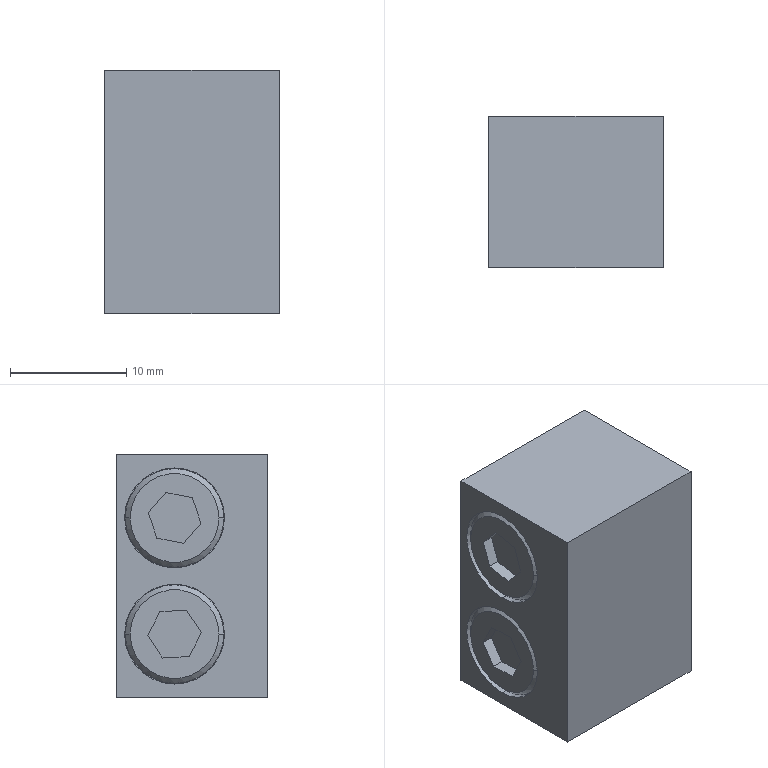Part | NX | 1 solid | 36 faces | box 15 x 13 x 21 mm | volume 4057 mm3 | plane 24 | cylinder 8 | cone 4 | commonest cylinder face diameters 8.5 x4 8.6 x4
STEP:
#1=CARTESIAN_POINT('',(-7.5,-2.325,5.));
#2=VERTEX_POINT('',#1);
#3=CARTESIAN_POINT('',(-7.5,5.325,5.));
#4=VERTEX_POINT('',#3);
#5=CARTESIAN_POINT('',(-7.5,1.5,5.));
#6=DIRECTION('',(-1.,0.,0.));
#7=DIRECTION('',(0.,0.,1.));
#8=AXIS2_PLACEMENT_3D('',#5,#6,#7);
#9=CIRCLE('',#8,3.825);
#10=EDGE_CURVE('',#2,#4,#9,.T.);
#11=ORIENTED_EDGE('',*,*,#10,.F.);
#12=CARTESIAN_POINT('',(-7.075,-2.75,5.));
#13=VERTEX_POINT('',#12);
#14=CARTESIAN_POINT('',(-7.5,-2.325,5.));
#15=DIRECTION('',(0.7071,-0.7071,0.));
#16=VECTOR('',#15,1000.);
#17=LINE('',#14,#16);
#18=EDGE_CURVE('',#13,#2,#17,.F.);
#19=ORIENTED_EDGE('',*,*,#18,.F.);
#20=CARTESIAN_POINT('',(-7.075,1.5,9.25));
#21=VERTEX_POINT('',#20);
#22=CARTESIAN_POINT('',(-7.075,1.5,5.));
#23=DIRECTION('',(1.,0.,0.));
#24=DIRECTION('',(0.,0.,1.));
#25=AXIS2_PLACEMENT_3D('',#22,#23,#24);
#26=CIRCLE('',#25,4.25);
#27=EDGE_CURVE('',#21,#13,#26,.T.);
#28=ORIENTED_EDGE('',*,*,#27,.F.);
#29=CARTESIAN_POINT('',(-7.075,5.75,5.));
#30=VERTEX_POINT('',#29);
#31=CARTESIAN_POINT('',(-7.075,1.5,5.));
#32=DIRECTION('',(1.,0.,0.));
#33=DIRECTION('',(0.,0.,1.));
#34=AXIS2_PLACEMENT_3D('',#31,#32,#33);
#35=CIRCLE('',#34,4.25);
#36=EDGE_CURVE('',#30,#21,#35,.T.);
#37=ORIENTED_EDGE('',*,*,#36,.F.);
#38=CARTESIAN_POINT('',(-7.5,5.325,5.));
#39=DIRECTION('',(0.7071,0.7071,0.));
#40=VECTOR('',#39,1000.);
#41=LINE('',#38,#40);
#42=EDGE_CURVE('',#30,#4,#41,.F.);
#43=ORIENTED_EDGE('',*,*,#42,.T.);
#44=EDGE_LOOP('',(#11,#19,#28,#37,#43));
#45=FACE_BOUND('',#44,.T.);
#46=CARTESIAN_POINT('',(-7.5,1.5,5.));
#47=DIRECTION('',(1.,0.,0.));
#48=DIRECTION('',(0.,-1.,0.));
#49=AXIS2_PLACEMENT_3D('',#46,#47,#48);
#50=CONICAL_SURFACE('',#49,3.825,0.7854);
#51=ADVANCED_FACE('',(#45),#50,.T.);
#52=CARTESIAN_POINT('',(-7.075,1.5,-0.75));
#53=VERTEX_POINT('',#52);
#54=CARTESIAN_POINT('',(-7.075,-2.75,-5.));
#55=VERTEX_POINT('',#54);
#56=CARTESIAN_POINT('',(-7.075,1.5,-5.));
#57=DIRECTION('',(1.,0.,0.));
#58=DIRECTION('',(0.,0.,1.));
#59=AXIS2_PLACEMENT_3D('',#56,#57,#58);
#60=CIRCLE('',#59,4.25);
#61=EDGE_CURVE('',#53,#55,#60,.T.);
#62=ORIENTED_EDGE('',*,*,#61,.F.);
#63=CARTESIAN_POINT('',(-7.075,5.75,-5.));
#64=VERTEX_POINT('',#63);
#65=CARTESIAN_POINT('',(-7.075,1.5,-5.));
#66=DIRECTION('',(1.,0.,0.));
#67=DIRECTION('',(0.,0.,1.));
#68=AXIS2_PLACEMENT_3D('',#65,#66,#67);
#69=CIRCLE('',#68,4.25);
#70=EDGE_CURVE('',#64,#53,#69,.T.);
#71=ORIENTED_EDGE('',*,*,#70,.F.);
#72=CARTESIAN_POINT('',(-7.5,5.325,-5.));
#73=VERTEX_POINT('',#72);
#74=CARTESIAN_POINT('',(-7.5,5.325,-5.));
#75=DIRECTION('',(0.7071,0.7071,0.));
#76=VECTOR('',#75,1000.);
#77=LINE('',#74,#76);
#78=EDGE_CURVE('',#64,#73,#77,.F.);
#79=ORIENTED_EDGE('',*,*,#78,.T.);
#80=CARTESIAN_POINT('',(-7.5,-2.325,-5.));
#81=VERTEX_POINT('',#80);
#82=CARTESIAN_POINT('',(-7.5,1.5,-5.));
#83=DIRECTION('',(-1.,0.,0.));
#84=DIRECTION('',(0.,0.,1.));
#85=AXIS2_PLACEMENT_3D('',#82,#83,#84);
#86=CIRCLE('',#85,3.825);
#87=EDGE_CURVE('',#81,#73,#86,.T.);
#88=ORIENTED_EDGE('',*,*,#87,.F.);
#89=CARTESIAN_POINT('',(-7.5,-2.325,-5.));
#90=DIRECTION('',(0.7071,-0.7071,0.));
#91=VECTOR('',#90,1000.);
#92=LINE('',#89,#91);
#93=EDGE_CURVE('',#55,#81,#92,.F.);
#94=ORIENTED_EDGE('',*,*,#93,.F.);
#95=EDGE_LOOP('',(#62,#71,#79,#88,#94));
#96=FACE_BOUND('',#95,.T.);
#97=CARTESIAN_POINT('',(-7.5,1.5,-5.));
#98=DIRECTION('',(1.,0.,0.));
#99=DIRECTION('',(0.,-1.,0.));
#100=AXIS2_PLACEMENT_3D('',#97,#98,#99);
#101=CONICAL_SURFACE('',#100,3.825,0.7854);
#102=ADVANCED_FACE('',(#96),#101,.T.);
#103=CARTESIAN_POINT('',(-5.5,1.5,9.25));
#104=VERTEX_POINT('',#103);
#105=CARTESIAN_POINT('',(-5.5,1.5,0.75));
#106=VERTEX_POINT('',#105);
#107=CARTESIAN_POINT('',(-5.5,1.5,5.));
#108=DIRECTION('',(-1.,0.,0.));
#109=DIRECTION('',(0.,0.,1.));
#110=AXIS2_PLACEMENT_3D('',#107,#108,#109);
#111=CIRCLE('',#110,4.25);
#112=EDGE_CURVE('',#104,#106,#111,.T.);
#113=ORIENTED_EDGE('',*,*,#112,.T.);
#114=CARTESIAN_POINT('',(-7.075,1.5,0.75));
#115=VERTEX_POINT('',#114);
#116=CARTESIAN_POINT('',(-7.5,1.5,0.75));
#117=DIRECTION('',(1.,0.,0.));
#118=VECTOR('',#117,1000.);
#119=LINE('',#116,#118);
#120=EDGE_CURVE('',#106,#115,#119,.F.);
#121=ORIENTED_EDGE('',*,*,#120,.T.);
#122=CARTESIAN_POINT('',(-7.075,1.5,5.));
#123=DIRECTION('',(1.,0.,0.));
#124=DIRECTION('',(0.,0.,1.));
#125=AXIS2_PLACEMENT_3D('',#122,#123,#124);
#126=CIRCLE('',#125,4.25);
#127=EDGE_CURVE('',#115,#30,#126,.T.);
#128=ORIENTED_EDGE('',*,*,#127,.T.);
#129=ORIENTED_EDGE('',*,*,#36,.T.);
#130=CARTESIAN_POINT('',(-7.5,1.5,9.25));
#131=DIRECTION('',(1.,0.,0.));
#132=VECTOR('',#131,1000.);
#133=LINE('',#130,#132);
#134=EDGE_CURVE('',#104,#21,#133,.F.);
#135=ORIENTED_EDGE('',*,*,#134,.F.);
#136=EDGE_LOOP('',(#113,#121,#128,#129,#135));
#137=FACE_BOUND('',#136,.T.);
#138=CARTESIAN_POINT('',(-7.5,1.5,5.));
#139=DIRECTION('',(1.,0.,0.));
#140=DIRECTION('',(0.,0.,-1.));
#141=AXIS2_PLACEMENT_3D('',#138,#139,#140);
#142=CYLINDRICAL_SURFACE('',#141,4.25);
#143=ADVANCED_FACE('',(#137),#142,.T.);
#144=ORIENTED_EDGE('',*,*,#61,.T.);
#145=CARTESIAN_POINT('',(-7.075,1.5,-9.25));
#146=VERTEX_POINT('',#145);
#147=CARTESIAN_POINT('',(-7.075,1.5,-5.));
#148=DIRECTION('',(1.,0.,0.));
#149=DIRECTION('',(0.,0.,1.));
#150=AXIS2_PLACEMENT_3D('',#147,#148,#149);
#151=CIRCLE('',#150,4.25);
#152=EDGE_CURVE('',#55,#146,#151,.T.);
#153=ORIENTED_EDGE('',*,*,#152,.T.);
#154=CARTESIAN_POINT('',(-5.5,1.5,-9.25));
#155=VERTEX_POINT('',#154);
#156=CARTESIAN_POINT('',(-7.5,1.5,-9.25));
#157=DIRECTION('',(1.,0.,0.));
#158=VECTOR('',#157,1000.);
#159=LINE('',#156,#158);
#160=EDGE_CURVE('',#155,#146,#159,.F.);
#161=ORIENTED_EDGE('',*,*,#160,.F.);
#162=CARTESIAN_POINT('',(-5.5,1.5,-0.75));
#163=VERTEX_POINT('',#162);
#164=CARTESIAN_POINT('',(-5.5,1.5,-5.));
#165=DIRECTION('',(-1.,0.,0.));
#166=DIRECTION('',(0.,0.,-1.));
#167=AXIS2_PLACEMENT_3D('',#164,#165,#166);
#168=CIRCLE('',#167,4.25);
#169=EDGE_CURVE('',#155,#163,#168,.T.);
#170=ORIENTED_EDGE('',*,*,#169,.T.);
#171=CARTESIAN_POINT('',(-7.5,1.5,-0.75));
#172=DIRECTION('',(1.,0.,0.));
#173=VECTOR('',#172,1000.);
#174=LINE('',#171,#173);
#175=EDGE_CURVE('',#163,#53,#174,.F.);
#176=ORIENTED_EDGE('',*,*,#175,.T.);
#177=EDGE_LOOP('',(#144,#153,#161,#170,#176));
#178=FACE_BOUND('',#177,.T.);
#179=CARTESIAN_POINT('',(-7.5,1.5,-5.));
#180=DIRECTION('',(1.,0.,0.));
#181=DIRECTION('',(0.,0.,-1.));
#182=AXIS2_PLACEMENT_3D('',#179,#180,#181);
#183=CYLINDRICAL_SURFACE('',#182,4.25);
#184=ADVANCED_FACE('',(#178),#183,.T.);
#185=CARTESIAN_POINT('',(-7.5,1.5,9.3));
#186=VERTEX_POINT('',#185);
#187=CARTESIAN_POINT('',(-7.5,1.5,0.7));
#188=VERTEX_POINT('',#187);
#189=CARTESIAN_POINT('',(-7.5,1.5,5.));
#190=DIRECTION('',(1.,0.,0.));
#191=DIRECTION('',(0.,0.,1.));
#192=AXIS2_PLACEMENT_3D('',#189,#190,#191);
#193=CIRCLE('',#192,4.3);
#194=EDGE_CURVE('',#186,#188,#193,.T.);
#195=ORIENTED_EDGE('',*,*,#194,.F.);
#196=CARTESIAN_POINT('',(-5.5,1.5,9.3));
#197=VERTEX_POINT('',#196);
#198=CARTESIAN_POINT('',(-5.5,1.5,9.3));
#199=DIRECTION('',(-1.,0.,0.));
#200=VECTOR('',#199,1000.);
#201=LINE('',#198,#200);
#202=EDGE_CURVE('',#197,#186,#201,.T.);
#203=ORIENTED_EDGE('',*,*,#202,.F.);
#204=CARTESIAN_POINT('',(-5.5,1.5,0.7));
#205=VERTEX_POINT('',#204);
#206=CARTESIAN_POINT('',(-5.5,1.5,5.));
#207=DIRECTION('',(1.,0.,0.));
#208=DIRECTION('',(0.,0.,1.));
#209=AXIS2_PLACEMENT_3D('',#206,#207,#208);
#210=CIRCLE('',#209,4.3);
#211=EDGE_CURVE('',#197,#205,#210,.T.);
#212=ORIENTED_EDGE('',*,*,#211,.T.);
#213=CARTESIAN_POINT('',(-5.5,1.5,0.7));
#214=DIRECTION('',(-1.,0.,0.));
#215=VECTOR('',#214,1000.);
#216=LINE('',#213,#215);
#217=EDGE_CURVE('',#205,#188,#216,.T.);
#218=ORIENTED_EDGE('',*,*,#217,.T.);
#219=EDGE_LOOP('',(#195,#203,#212,#218));
#220=FACE_BOUND('',#219,.T.);
#221=CARTESIAN_POINT('',(-5.5,1.5,5.));
#222=DIRECTION('',(-1.,0.,0.));
#223=DIRECTION('',(0.,0.,1.));
#224=AXIS2_PLACEMENT_3D('',#221,#222,#223);
#225=CYLINDRICAL_SURFACE('',#224,4.3);
#226=ADVANCED_FACE('',(#220),#225,.F.);
#227=CARTESIAN_POINT('',(-5.5,1.5,-0.7));
#228=VERTEX_POINT('',#227);
#229=CARTESIAN_POINT('',(-5.5,1.5,-9.3));
#230=VERTEX_POINT('',#229);
#231=CARTESIAN_POINT('',(-5.5,1.5,-5.));
#232=DIRECTION('',(1.,0.,0.));
#233=DIRECTION('',(0.,0.,-1.));
#234=AXIS2_PLACEMENT_3D('',#231,#232,#233);
#235=CIRCLE('',#234,4.3);
#236=EDGE_CURVE('',#228,#230,#235,.T.);
#237=ORIENTED_EDGE('',*,*,#236,.T.);
#238=CARTESIAN_POINT('',(-7.5,1.5,-9.3));
#239=VERTEX_POINT('',#238);
#240=CARTESIAN_POINT('',(-5.5,1.5,-9.3));
#241=DIRECTION('',(-1.,0.,0.));
#242=VECTOR('',#241,1000.);
#243=LINE('',#240,#242);
#244=EDGE_CURVE('',#239,#230,#243,.F.);
#245=ORIENTED_EDGE('',*,*,#244,.F.);
#246=CARTESIAN_POINT('',(-7.5,1.5,-0.7));
#247=VERTEX_POINT('',#246);
#248=CARTESIAN_POINT('',(-7.5,1.5,-5.));
#249=DIRECTION('',(1.,0.,0.));
#250=DIRECTION('',(0.,0.,-1.));
#251=AXIS2_PLACEMENT_3D('',#248,#249,#250);
#252=CIRCLE('',#251,4.3);
#253=EDGE_CURVE('',#247,#239,#252,.T.);
#254=ORIENTED_EDGE('',*,*,#253,.F.);
#255=CARTESIAN_POINT('',(-5.5,1.5,-0.7));
#256=DIRECTION('',(-1.,0.,0.));
#257=VECTOR('',#256,1000.);
#258=LINE('',#255,#257);
#259=EDGE_CURVE('',#247,#228,#258,.F.);
#260=ORIENTED_EDGE('',*,*,#259,.T.);
#261=EDGE_LOOP('',(#237,#245,#254,#260));
#262=FACE_BOUND('',#261,.T.);
#263=CARTESIAN_POINT('',(-5.5,1.5,-5.));
#264=DIRECTION('',(-1.,0.,0.));
#265=DIRECTION('',(0.,0.,1.));
#266=AXIS2_PLACEMENT_3D('',#263,#264,#265);
#267=CYLINDRICAL_SURFACE('',#266,4.3);
#268=ADVANCED_FACE('',(#262),#267,.F.);
#269=CARTESIAN_POINT('',(-5.5,1.5,5.));
#270=DIRECTION('',(1.,0.,0.));
#271=DIRECTION('',(0.,0.,1.));
#272=AXIS2_PLACEMENT_3D('',#269,#270,#271);
#273=CIRCLE('',#272,4.3);
#274=EDGE_CURVE('',#205,#197,#273,.T.);
#275=ORIENTED_EDGE('',*,*,#274,.F.);
#276=ORIENTED_EDGE('',*,*,#211,.F.);
#277=EDGE_LOOP('',(#275,#276));
#278=FACE_BOUND('',#277,.T.);
#279=ORIENTED_EDGE('',*,*,#112,.F.);
#280=CARTESIAN_POINT('',(-5.5,1.5,5.));
#281=DIRECTION('',(-1.,0.,0.));
#282=DIRECTION('',(0.,0.,1.));
#283=AXIS2_PLACEMENT_3D('',#280,#281,#282);
#284=CIRCLE('',#283,4.25);
#285=EDGE_CURVE('',#106,#104,#284,.T.);
#286=ORIENTED_EDGE('',*,*,#285,.F.);
#287=EDGE_LOOP('',(#279,#286));
#288=FACE_BOUND('',#287,.T.);
#289=CARTESIAN_POINT('',(-5.5,1.5,5.));
#290=DIRECTION('',(-1.,0.,0.));
#291=DIRECTION('',(0.,0.,1.));
#292=AXIS2_PLACEMENT_3D('',#289,#290,#291);
#293=PLANE('',#292);
#294=ADVANCED_FACE('',(#278,#288),#293,.T.);
#295=ORIENTED_EDGE('',*,*,#236,.F.);
#296=CARTESIAN_POINT('',(-5.5,1.5,-5.));
#297=DIRECTION('',(1.,0.,0.));
#298=DIRECTION('',(0.,0.,-1.));
#299=AXIS2_PLACEMENT_3D('',#296,#297,#298);
#300=CIRCLE('',#299,4.3);
#301=EDGE_CURVE('',#230,#228,#300,.T.);
#302=ORIENTED_EDGE('',*,*,#301,.F.);
#303=EDGE_LOOP('',(#295,#302));
#304=FACE_BOUND('',#303,.T.);
#305=CARTESIAN_POINT('',(-5.5,1.5,-5.));
#306=DIRECTION('',(-1.,0.,0.));
#307=DIRECTION('',(0.,0.,-1.));
#308=AXIS2_PLACEMENT_3D('',#305,#306,#307);
#309=CIRCLE('',#308,4.25);
#310=EDGE_CURVE('',#163,#155,#309,.T.);
#311=ORIENTED_EDGE('',*,*,#310,.F.);
#312=ORIENTED_EDGE('',*,*,#169,.F.);
#313=EDGE_LOOP('',(#311,#312));
#314=FACE_BOUND('',#313,.T.);
#315=CARTESIAN_POINT('',(-5.5,1.5,-5.));
#316=DIRECTION('',(1.,0.,0.));
#317=DIRECTION('',(0.,1.,0.));
#318=AXIS2_PLACEMENT_3D('',#315,#316,#317);
#319=PLANE('',#318);
#320=ADVANCED_FACE('',(#304,#314),#319,.F.);
#321=CARTESIAN_POINT('',(-7.5,6.5,-10.5));
#322=VERTEX_POINT('',#321);
#323=CARTESIAN_POINT('',(-7.5,-6.5,-10.5));
#324=VERTEX_POINT('',#323);
#325=CARTESIAN_POINT('',(-7.5,6.5,-10.5));
#326=DIRECTION('',(0.,-1.,0.));
#327=VECTOR('',#326,1000.);
#328=LINE('',#325,#327);
#329=EDGE_CURVE('',#322,#324,#328,.T.);
#330=ORIENTED_EDGE('',*,*,#329,.T.);
#331=CARTESIAN_POINT('',(-7.5,-6.5,10.5));
#332=VERTEX_POINT('',#331);
#333=CARTESIAN_POINT('',(-7.5,-6.5,10.5));
#334=DIRECTION('',(0.,0.,-1.));
#335=VECTOR('',#334,1000.);
#336=LINE('',#333,#335);
#337=EDGE_CURVE('',#332,#324,#336,.T.);
#338=ORIENTED_EDGE('',*,*,#337,.F.);
#339=CARTESIAN_POINT('',(-7.5,6.5,10.5));
#340=VERTEX_POINT('',#339);
#341=CARTESIAN_POINT('',(-7.5,6.5,10.5));
#342=DIRECTION('',(0.,-1.,0.));
#343=VECTOR('',#342,1000.);
#344=LINE('',#341,#343);
#345=EDGE_CURVE('',#340,#332,#344,.T.);
#346=ORIENTED_EDGE('',*,*,#345,.F.);
#347=CARTESIAN_POINT('',(-7.5,6.5,10.5));
#348=DIRECTION('',(0.,0.,-1.));
#349=VECTOR('',#348,1000.);
#350=LINE('',#347,#349);
#351=EDGE_CURVE('',#340,#322,#350,.T.);
#352=ORIENTED_EDGE('',*,*,#351,.T.);
#353=EDGE_LOOP('',(#330,#338,#346,#352));
#354=FACE_BOUND('',#353,.T.);
#355=CARTESIAN_POINT('',(-7.5,1.5,-5.));
#356=DIRECTION('',(1.,0.,0.));
#357=DIRECTION('',(0.,0.,-1.));
#358=AXIS2_PLACEMENT_3D('',#355,#356,#357);
#359=CIRCLE('',#358,4.3);
#360=EDGE_CURVE('',#239,#247,#359,.T.);
#361=ORIENTED_EDGE('',*,*,#360,.T.);
#362=ORIENTED_EDGE('',*,*,#253,.T.);
#363=EDGE_LOOP('',(#361,#362));
#364=FACE_BOUND('',#363,.T.);
#365=ORIENTED_EDGE('',*,*,#194,.T.);
#366=CARTESIAN_POINT('',(-7.5,1.5,5.));
#367=DIRECTION('',(1.,0.,0.));
#368=DIRECTION('',(0.,0.,1.));
#369=AXIS2_PLACEMENT_3D('',#366,#367,#368);
#370=CIRCLE('',#369,4.3);
#371=EDGE_CURVE('',#188,#186,#370,.T.);
#372=ORIENTED_EDGE('',*,*,#371,.T.);
#373=EDGE_LOOP('',(#365,#372));
#374=FACE_BOUND('',#373,.T.);
#375=CARTESIAN_POINT('',(-7.5,6.5,10.5));
#376=DIRECTION('',(1.,0.,0.));
#377=DIRECTION('',(0.,1.,0.));
#378=AXIS2_PLACEMENT_3D('',#375,#376,#377);
#379=PLANE('',#378);
#380=ADVANCED_FACE('',(#354,#364,#374),#379,.F.);
#381=CARTESIAN_POINT('',(7.5,-6.5,-10.5));
#382=VERTEX_POINT('',#381);
#383=CARTESIAN_POINT('',(-7.5,-6.5,-10.5));
#384=DIRECTION('',(1.,0.,0.));
#385=VECTOR('',#384,1000.);
#386=LINE('',#383,#385);
#387=EDGE_CURVE('',#324,#382,#386,.T.);
#388=ORIENTED_EDGE('',*,*,#387,.T.);
#389=CARTESIAN_POINT('',(7.5,-6.5,10.5));
#390=VERTEX_POINT('',#389);
#391=CARTESIAN_POINT('',(7.5,-6.5,10.5));
#392=DIRECTION('',(0.,0.,-1.));
#393=VECTOR('',#392,1000.);
#394=LINE('',#391,#393);
#395=EDGE_CURVE('',#390,#382,#394,.T.);
#396=ORIENTED_EDGE('',*,*,#395,.F.);
#397=CARTESIAN_POINT('',(-7.5,-6.5,10.5));
#398=DIRECTION('',(1.,0.,0.));
#399=VECTOR('',#398,1000.);
#400=LINE('',#397,#399);
#401=EDGE_CURVE('',#332,#390,#400,.T.);
#402=ORIENTED_EDGE('',*,*,#401,.F.);
#403=ORIENTED_EDGE('',*,*,#337,.T.);
#404=EDGE_LOOP('',(#388,#396,#402,#403));
#405=FACE_BOUND('',#404,.T.);
#406=CARTESIAN_POINT('',(-7.5,-6.5,10.5));
#407=DIRECTION('',(0.,1.,0.));
#408=DIRECTION('',(1.,0.,0.));
#409=AXIS2_PLACEMENT_3D('',#406,#407,#408);
#410=PLANE('',#409);
#411=ADVANCED_FACE('',(#405),#410,.F.);
#412=CARTESIAN_POINT('',(7.5,6.5,-10.5));
#413=VERTEX_POINT('',#412);
#414=CARTESIAN_POINT('',(7.5,6.5,-10.5));
#415=DIRECTION('',(0.,1.,0.));
#416=VECTOR('',#415,1000.);
#417=LINE('',#414,#416);
#418=EDGE_CURVE('',#382,#413,#417,.T.);
#419=ORIENTED_EDGE('',*,*,#418,.T.);
#420=CARTESIAN_POINT('',(7.5,6.5,10.5));
#421=VERTEX_POINT('',#420);
#422=CARTESIAN_POINT('',(7.5,6.5,10.5));
#423=DIRECTION('',(0.,0.,-1.));
#424=VECTOR('',#423,1000.);
#425=LINE('',#422,#424);
#426=EDGE_CURVE('',#421,#413,#425,.T.);
#427=ORIENTED_EDGE('',*,*,#426,.F.);
#428=CARTESIAN_POINT('',(7.5,6.5,10.5));
#429=DIRECTION('',(0.,1.,0.));
#430=VECTOR('',#429,1000.);
#431=LINE('',#428,#430);
#432=EDGE_CURVE('',#390,#421,#431,.T.);
#433=ORIENTED_EDGE('',*,*,#432,.F.);
#434=ORIENTED_EDGE('',*,*,#395,.T.);
#435=EDGE_LOOP('',(#419,#427,#433,#434));
#436=FACE_BOUND('',#435,.T.);
#437=CARTESIAN_POINT('',(7.5,6.5,10.5));
#438=DIRECTION('',(-1.,0.,0.));
#439=DIRECTION('',(0.,1.,0.));
#440=AXIS2_PLACEMENT_3D('',#437,#438,#439);
#441=PLANE('',#440);
#442=ADVANCED_FACE('',(#436),#441,.F.);
#443=CARTESIAN_POINT('',(-7.5,6.5,-10.5));
#444=DIRECTION('',(-1.,0.,0.));
#445=VECTOR('',#444,1000.);
#446=LINE('',#443,#445);
#447=EDGE_CURVE('',#413,#322,#446,.T.);
#448=ORIENTED_EDGE('',*,*,#447,.T.);
#449=ORIENTED_EDGE('',*,*,#351,.F.);
#450=CARTESIAN_POINT('',(-7.5,6.5,10.5));
#451=DIRECTION('',(-1.,0.,0.));
#452=VECTOR('',#451,1000.);
#453=LINE('',#450,#452);
#454=EDGE_CURVE('',#421,#340,#453,.T.);
#455=ORIENTED_EDGE('',*,*,#454,.F.);
#456=ORIENTED_EDGE('',*,*,#426,.T.);
#457=EDGE_LOOP('',(#448,#449,#455,#456));
#458=FACE_BOUND('',#457,.T.);
#459=CARTESIAN_POINT('',(-7.5,6.5,10.5));
#460=DIRECTION('',(0.,-1.,0.));
#461=DIRECTION('',(0.,0.,-1.));
#462=AXIS2_PLACEMENT_3D('',#459,#460,#461);
#463=PLANE('',#462);
#464=ADVANCED_FACE('',(#458),#463,.F.);
#465=ORIENTED_EDGE('',*,*,#345,.T.);
#466=ORIENTED_EDGE('',*,*,#401,.T.);
#467=ORIENTED_EDGE('',*,*,#432,.T.);
#468=ORIENTED_EDGE('',*,*,#454,.T.);
#469=EDGE_LOOP('',(#465,#466,#467,#468));
#470=FACE_BOUND('',#469,.T.);
#471=CARTESIAN_POINT('',(-7.5,-6.5,10.5));
#472=DIRECTION('',(0.,0.,1.));
#473=DIRECTION('',(1.,0.,0.));
#474=AXIS2_PLACEMENT_3D('',#471,#472,#473);
#475=PLANE('',#474);
#476=ADVANCED_FACE('',(#470),#475,.T.);
#477=ORIENTED_EDGE('',*,*,#329,.F.);
#478=ORIENTED_EDGE('',*,*,#447,.F.);
#479=ORIENTED_EDGE('',*,*,#418,.F.);
#480=ORIENTED_EDGE('',*,*,#387,.F.);
#481=EDGE_LOOP('',(#477,#478,#479,#480));
#482=FACE_BOUND('',#481,.T.);
#483=CARTESIAN_POINT('',(-7.5,-6.5,-10.5));
#484=DIRECTION('',(0.,0.,1.));
#485=DIRECTION('',(1.,0.,0.));
#486=AXIS2_PLACEMENT_3D('',#483,#484,#485);
#487=PLANE('',#486);
#488=ADVANCED_FACE('',(#482),#487,.F.);
#489=CARTESIAN_POINT('',(-7.5,3.766,5.446));
#490=VERTEX_POINT('',#489);
#491=CARTESIAN_POINT('',(-7.5,3.019,3.261));
#492=VERTEX_POINT('',#491);
#493=CARTESIAN_POINT('',(-7.5,3.766,5.446));
#494=DIRECTION('',(0.,-0.3232,-0.9463));
#495=VECTOR('',#494,1000.);
#496=LINE('',#493,#495);
#497=EDGE_CURVE('',#490,#492,#496,.T.);
#498=ORIENTED_EDGE('',*,*,#497,.T.);
#499=CARTESIAN_POINT('',(-6.5,3.019,3.261));
#500=VERTEX_POINT('',#499);
#501=CARTESIAN_POINT('',(-6.5,3.019,3.261));
#502=DIRECTION('',(-1.,0.,0.));
#503=VECTOR('',#502,1000.);
#504=LINE('',#501,#503);
#505=EDGE_CURVE('',#500,#492,#504,.T.);
#506=ORIENTED_EDGE('',*,*,#505,.F.);
#507=CARTESIAN_POINT('',(-6.5,3.766,5.446));
#508=VERTEX_POINT('',#507);
#509=CARTESIAN_POINT('',(-6.5,3.766,5.446));
#510=DIRECTION('',(0.,-0.3232,-0.9463));
#511=VECTOR('',#510,1000.);
#512=LINE('',#509,#511);
#513=EDGE_CURVE('',#508,#500,#512,.T.);
#514=ORIENTED_EDGE('',*,*,#513,.F.);
#515=CARTESIAN_POINT('',(-6.5,3.766,5.446));
#516=DIRECTION('',(-1.,0.,0.));
#517=VECTOR('',#516,1000.);
#518=LINE('',#515,#517);
#519=EDGE_CURVE('',#508,#490,#518,.T.);
#520=ORIENTED_EDGE('',*,*,#519,.T.);
#521=EDGE_LOOP('',(#498,#506,#514,#520));
#522=FACE_BOUND('',#521,.T.);
#523=CARTESIAN_POINT('',(-6.5,3.766,5.446));
#524=DIRECTION('',(0.,0.9463,-0.3232));
#525=DIRECTION('',(-1.,0.,0.));
#526=AXIS2_PLACEMENT_3D('',#523,#524,#525);
#527=PLANE('',#526);
#528=ADVANCED_FACE('',(#522),#527,.F.);
#529=CARTESIAN_POINT('',(-7.5,0.7535,2.815));
#530=VERTEX_POINT('',#529);
#531=CARTESIAN_POINT('',(-7.5,-0.7659,4.554));
#532=VERTEX_POINT('',#531);
#533=CARTESIAN_POINT('',(-7.5,0.7535,2.815));
#534=DIRECTION('',(0.,-0.6579,0.7531));
#535=VECTOR('',#534,1000.);
#536=LINE('',#533,#535);
#537=EDGE_CURVE('',#530,#532,#536,.T.);
#538=ORIENTED_EDGE('',*,*,#537,.T.);
#539=CARTESIAN_POINT('',(-6.5,-0.7659,4.554));
#540=VERTEX_POINT('',#539);
#541=CARTESIAN_POINT('',(-6.5,-0.7659,4.554));
#542=DIRECTION('',(-1.,0.,0.));
#543=VECTOR('',#542,1000.);
#544=LINE('',#541,#543);
#545=EDGE_CURVE('',#540,#532,#544,.T.);
#546=ORIENTED_EDGE('',*,*,#545,.F.);
#547=CARTESIAN_POINT('',(-6.5,0.7535,2.815));
#548=VERTEX_POINT('',#547);
#549=CARTESIAN_POINT('',(-6.5,0.7535,2.815));
#550=DIRECTION('',(0.,-0.6579,0.7531));
#551=VECTOR('',#550,1000.);
#552=LINE('',#549,#551);
#553=EDGE_CURVE('',#548,#540,#552,.T.);
#554=ORIENTED_EDGE('',*,*,#553,.F.);
#555=CARTESIAN_POINT('',(-6.5,0.7535,2.815));
#556=DIRECTION('',(-1.,0.,0.));
#557=VECTOR('',#556,1000.);
#558=LINE('',#555,#557);
#559=EDGE_CURVE('',#548,#530,#558,.T.);
#560=ORIENTED_EDGE('',*,*,#559,.T.);
#561=EDGE_LOOP('',(#538,#546,#554,#560));
#562=FACE_BOUND('',#561,.T.);
#563=CARTESIAN_POINT('',(-6.5,0.7535,2.815));
#564=DIRECTION('',(0.,-0.7531,-0.6579));
#565=DIRECTION('',(0.,0.6579,-0.7531));
#566=AXIS2_PLACEMENT_3D('',#563,#564,#565);
#567=PLANE('',#566);
#568=ADVANCED_FACE('',(#562),#567,.F.);
#569=CARTESIAN_POINT('',(-6.5,-0.01938,6.739));
#570=VERTEX_POINT('',#569);
#571=CARTESIAN_POINT('',(-6.5,-0.7659,4.554));
#572=DIRECTION('',(0.,0.3232,0.9463));
#573=VECTOR('',#572,1000.);
#574=LINE('',#571,#573);
#575=EDGE_CURVE('',#540,#570,#574,.T.);
#576=ORIENTED_EDGE('',*,*,#575,.T.);
#577=CARTESIAN_POINT('',(-6.5,2.246,7.185));
#578=VERTEX_POINT('',#577);
#579=CARTESIAN_POINT('',(-6.5,-0.01938,6.739));
#580=DIRECTION('',(0.,0.9812,0.1932));
#581=VECTOR('',#580,1000.);
#582=LINE('',#579,#581);
#583=EDGE_CURVE('',#570,#578,#582,.T.);
#584=ORIENTED_EDGE('',*,*,#583,.T.);
#585=CARTESIAN_POINT('',(-6.5,2.246,7.185));
#586=DIRECTION('',(0.,0.6579,-0.7531));
#587=VECTOR('',#586,1000.);
#588=LINE('',#585,#587);
#589=EDGE_CURVE('',#578,#508,#588,.T.);
#590=ORIENTED_EDGE('',*,*,#589,.T.);
#591=ORIENTED_EDGE('',*,*,#513,.T.);
#592=CARTESIAN_POINT('',(-6.5,3.019,3.261));
#593=DIRECTION('',(0.,-0.9812,-0.1932));
#594=VECTOR('',#593,1000.);
#595=LINE('',#592,#594);
#596=EDGE_CURVE('',#500,#548,#595,.T.);
#597=ORIENTED_EDGE('',*,*,#596,.T.);
#598=ORIENTED_EDGE('',*,*,#553,.T.);
#599=EDGE_LOOP('',(#576,#584,#590,#591,#597,#598));
#600=FACE_BOUND('',#599,.T.);
#601=CARTESIAN_POINT('',(-6.5,-0.7659,4.554));
#602=DIRECTION('',(1.,0.,0.));
#603=DIRECTION('',(0.,1.,0.));
#604=AXIS2_PLACEMENT_3D('',#601,#602,#603);
#605=PLANE('',#604);
#606=ADVANCED_FACE('',(#600),#605,.F.);
#607=ORIENTED_EDGE('',*,*,#87,.T.);
#608=CARTESIAN_POINT('',(-7.5,1.5,-5.));
#609=DIRECTION('',(-1.,0.,0.));
#610=DIRECTION('',(0.,0.,1.));
#611=AXIS2_PLACEMENT_3D('',#608,#609,#610);
#612=CIRCLE('',#611,3.825);
#613=EDGE_CURVE('',#73,#81,#612,.T.);
#614=ORIENTED_EDGE('',*,*,#613,.T.);
#615=EDGE_LOOP('',(#607,#614));
#616=FACE_BOUND('',#615,.T.);
#617=CARTESIAN_POINT('',(-7.5,0.2336,-6.931));
#618=VERTEX_POINT('',#617);
#619=CARTESIAN_POINT('',(-7.5,-0.8057,-4.869));
#620=VERTEX_POINT('',#619);
#621=CARTESIAN_POINT('',(-7.5,0.2336,-6.931));
#622=DIRECTION('',(0.,-0.45,0.893));
#623=VECTOR('',#622,1000.);
#624=LINE('',#621,#623);
#625=EDGE_CURVE('',#618,#620,#624,.T.);
#626=ORIENTED_EDGE('',*,*,#625,.F.);
#627=CARTESIAN_POINT('',(-7.5,2.539,-7.062));
#628=VERTEX_POINT('',#627);
#629=CARTESIAN_POINT('',(-7.5,2.539,-7.062));
#630=DIRECTION('',(0.,-0.9984,0.05679));
#631=VECTOR('',#630,1000.);
#632=LINE('',#629,#631);
#633=EDGE_CURVE('',#628,#618,#632,.T.);
#634=ORIENTED_EDGE('',*,*,#633,.F.);
#635=CARTESIAN_POINT('',(-7.5,3.806,-5.131));
#636=VERTEX_POINT('',#635);
#637=CARTESIAN_POINT('',(-7.5,3.806,-5.131));
#638=DIRECTION('',(0.,-0.5484,-0.8362));
#639=VECTOR('',#638,1000.);
#640=LINE('',#637,#639);
#641=EDGE_CURVE('',#636,#628,#640,.T.);
#642=ORIENTED_EDGE('',*,*,#641,.F.);
#643=CARTESIAN_POINT('',(-7.5,2.766,-3.069));
#644=VERTEX_POINT('',#643);
#645=CARTESIAN_POINT('',(-7.5,2.766,-3.069));
#646=DIRECTION('',(0.,0.45,-0.893));
#647=VECTOR('',#646,1000.);
#648=LINE('',#645,#647);
#649=EDGE_CURVE('',#644,#636,#648,.T.);
#650=ORIENTED_EDGE('',*,*,#649,.F.);
#651=CARTESIAN_POINT('',(-7.5,0.4607,-2.938));
#652=VERTEX_POINT('',#651);
#653=CARTESIAN_POINT('',(-7.5,0.4607,-2.938));
#654=DIRECTION('',(0.,0.9984,-0.05679));
#655=VECTOR('',#654,1000.);
#656=LINE('',#653,#655);
#657=EDGE_CURVE('',#652,#644,#656,.T.);
#658=ORIENTED_EDGE('',*,*,#657,.F.);
#659=CARTESIAN_POINT('',(-7.5,-0.8057,-4.869));
#660=DIRECTION('',(0.,0.5484,0.8362));
#661=VECTOR('',#660,1000.);
#662=LINE('',#659,#661);
#663=EDGE_CURVE('',#620,#652,#662,.T.);
#664=ORIENTED_EDGE('',*,*,#663,.F.);
#665=EDGE_LOOP('',(#626,#634,#642,#650,#658,#664));
#666=FACE_BOUND('',#665,.T.);
#667=CARTESIAN_POINT('',(-7.5,1.5,-5.));
#668=DIRECTION('',(-1.,0.,0.));
#669=DIRECTION('',(0.,0.,1.));
#670=AXIS2_PLACEMENT_3D('',#667,#668,#669);
#671=PLANE('',#670);
#672=ADVANCED_FACE('',(#616,#666),#671,.T.);
#673=CARTESIAN_POINT('',(-7.5,2.246,7.185));
#674=VERTEX_POINT('',#673);
#675=CARTESIAN_POINT('',(-7.5,2.246,7.185));
#676=DIRECTION('',(0.,0.6579,-0.7531));
#677=VECTOR('',#676,1000.);
#678=LINE('',#675,#677);
#679=EDGE_CURVE('',#674,#490,#678,.T.);
#680=ORIENTED_EDGE('',*,*,#679,.T.);
#681=ORIENTED_EDGE('',*,*,#519,.F.);
#682=ORIENTED_EDGE('',*,*,#589,.F.);
#683=CARTESIAN_POINT('',(-6.5,2.246,7.185));
#684=DIRECTION('',(-1.,0.,0.));
#685=VECTOR('',#684,1000.);
#686=LINE('',#683,#685);
#687=EDGE_CURVE('',#578,#674,#686,.T.);
#688=ORIENTED_EDGE('',*,*,#687,.T.);
#689=EDGE_LOOP('',(#680,#681,#682,#688));
#690=FACE_BOUND('',#689,.T.);
#691=CARTESIAN_POINT('',(-6.5,2.246,7.185));
#692=DIRECTION('',(0.,0.7531,0.6579));
#693=DIRECTION('',(1.,0.,0.));
#694=AXIS2_PLACEMENT_3D('',#691,#692,#693);
#695=PLANE('',#694);
#696=ADVANCED_FACE('',(#690),#695,.F.);
#697=ORIENTED_EDGE('',*,*,#10,.T.);
#698=CARTESIAN_POINT('',(-7.5,1.5,5.));
#699=DIRECTION('',(-1.,0.,0.));
#700=DIRECTION('',(0.,0.,1.));
#701=AXIS2_PLACEMENT_3D('',#698,#699,#700);
#702=CIRCLE('',#701,3.825);
#703=EDGE_CURVE('',#4,#2,#702,.T.);
#704=ORIENTED_EDGE('',*,*,#703,.T.);
#705=EDGE_LOOP('',(#697,#704));
#706=FACE_BOUND('',#705,.T.);
#707=CARTESIAN_POINT('',(-7.5,-0.01938,6.739));
#708=VERTEX_POINT('',#707);
#709=CARTESIAN_POINT('',(-7.5,-0.7659,4.554));
#710=DIRECTION('',(0.,0.3232,0.9463));
#711=VECTOR('',#710,1000.);
#712=LINE('',#709,#711);
#713=EDGE_CURVE('',#532,#708,#712,.T.);
#714=ORIENTED_EDGE('',*,*,#713,.F.);
#715=ORIENTED_EDGE('',*,*,#537,.F.);
#716=CARTESIAN_POINT('',(-7.5,3.019,3.261));
#717=DIRECTION('',(0.,-0.9812,-0.1932));
#718=VECTOR('',#717,1000.);
#719=LINE('',#716,#718);
#720=EDGE_CURVE('',#492,#530,#719,.T.);
#721=ORIENTED_EDGE('',*,*,#720,.F.);
#722=ORIENTED_EDGE('',*,*,#497,.F.);
#723=ORIENTED_EDGE('',*,*,#679,.F.);
#724=CARTESIAN_POINT('',(-7.5,-0.01938,6.739));
#725=DIRECTION('',(0.,0.9812,0.1932));
#726=VECTOR('',#725,1000.);
#727=LINE('',#724,#726);
#728=EDGE_CURVE('',#708,#674,#727,.T.);
#729=ORIENTED_EDGE('',*,*,#728,.F.);
#730=EDGE_LOOP('',(#714,#715,#721,#722,#723,#729));
#731=FACE_BOUND('',#730,.T.);
#732=CARTESIAN_POINT('',(-7.5,1.5,5.));
#733=DIRECTION('',(-1.,0.,0.));
#734=DIRECTION('',(0.,0.,1.));
#735=AXIS2_PLACEMENT_3D('',#732,#733,#734);
#736=PLANE('',#735);
#737=ADVANCED_FACE('',(#706,#731),#736,.T.);
#738=ORIENTED_EDGE('',*,*,#720,.T.);
#739=ORIENTED_EDGE('',*,*,#559,.F.);
#740=ORIENTED_EDGE('',*,*,#596,.F.);
#741=ORIENTED_EDGE('',*,*,#505,.T.);
#742=EDGE_LOOP('',(#738,#739,#740,#741));
#743=FACE_BOUND('',#742,.T.);
#744=CARTESIAN_POINT('',(-6.5,3.019,3.261));
#745=DIRECTION('',(0.,0.1932,-0.9812));
#746=DIRECTION('',(-1.,0.,0.));
#747=AXIS2_PLACEMENT_3D('',#744,#745,#746);
#748=PLANE('',#747);
#749=ADVANCED_FACE('',(#743),#748,.F.);
#750=ORIENTED_EDGE('',*,*,#728,.T.);
#751=ORIENTED_EDGE('',*,*,#687,.F.);
#752=ORIENTED_EDGE('',*,*,#583,.F.);
#753=CARTESIAN_POINT('',(-6.5,-0.01938,6.739));
#754=DIRECTION('',(-1.,0.,0.));
#755=VECTOR('',#754,1000.);
#756=LINE('',#753,#755);
#757=EDGE_CURVE('',#570,#708,#756,.T.);
#758=ORIENTED_EDGE('',*,*,#757,.T.);
#759=EDGE_LOOP('',(#750,#751,#752,#758));
#760=FACE_BOUND('',#759,.T.);
#761=CARTESIAN_POINT('',(-6.5,-0.01938,6.739));
#762=DIRECTION('',(0.,-0.1932,0.9812));
#763=DIRECTION('',(-1.,0.,0.));
#764=AXIS2_PLACEMENT_3D('',#761,#762,#763);
#765=PLANE('',#764);
#766=ADVANCED_FACE('',(#760),#765,.F.);
#767=ORIENTED_EDGE('',*,*,#625,.T.);
#768=CARTESIAN_POINT('',(-6.5,-0.8057,-4.869));
#769=VERTEX_POINT('',#768);
#770=CARTESIAN_POINT('',(-6.5,-0.8057,-4.869));
#771=DIRECTION('',(-1.,0.,0.));
#772=VECTOR('',#771,1000.);
#773=LINE('',#770,#772);
#774=EDGE_CURVE('',#769,#620,#773,.T.);
#775=ORIENTED_EDGE('',*,*,#774,.F.);
#776=CARTESIAN_POINT('',(-6.5,0.2336,-6.931));
#777=VERTEX_POINT('',#776);
#778=CARTESIAN_POINT('',(-6.5,0.2336,-6.931));
#779=DIRECTION('',(0.,-0.45,0.893));
#780=VECTOR('',#779,1000.);
#781=LINE('',#778,#780);
#782=EDGE_CURVE('',#777,#769,#781,.T.);
#783=ORIENTED_EDGE('',*,*,#782,.F.);
#784=CARTESIAN_POINT('',(-6.5,0.2336,-6.931));
#785=DIRECTION('',(-1.,0.,0.));
#786=VECTOR('',#785,1000.);
#787=LINE('',#784,#786);
#788=EDGE_CURVE('',#777,#618,#787,.T.);
#789=ORIENTED_EDGE('',*,*,#788,.T.);
#790=EDGE_LOOP('',(#767,#775,#783,#789));
#791=FACE_BOUND('',#790,.T.);
#792=CARTESIAN_POINT('',(-6.5,0.2336,-6.931));
#793=DIRECTION('',(0.,-0.893,-0.45));
#794=DIRECTION('',(0.,0.45,-0.893));
#795=AXIS2_PLACEMENT_3D('',#792,#793,#794);
#796=PLANE('',#795);
#797=ADVANCED_FACE('',(#791),#796,.F.);
#798=ORIENTED_EDGE('',*,*,#633,.T.);
#799=ORIENTED_EDGE('',*,*,#788,.F.);
#800=CARTESIAN_POINT('',(-6.5,2.539,-7.062));
#801=VERTEX_POINT('',#800);
#802=CARTESIAN_POINT('',(-6.5,2.539,-7.062));
#803=DIRECTION('',(0.,-0.9984,0.05679));
#804=VECTOR('',#803,1000.);
#805=LINE('',#802,#804);
#806=EDGE_CURVE('',#801,#777,#805,.T.);
#807=ORIENTED_EDGE('',*,*,#806,.F.);
#808=CARTESIAN_POINT('',(-6.5,2.539,-7.062));
#809=DIRECTION('',(-1.,0.,0.));
#810=VECTOR('',#809,1000.);
#811=LINE('',#808,#810);
#812=EDGE_CURVE('',#801,#628,#811,.T.);
#813=ORIENTED_EDGE('',*,*,#812,.T.);
#814=EDGE_LOOP('',(#798,#799,#807,#813));
#815=FACE_BOUND('',#814,.T.);
#816=CARTESIAN_POINT('',(-6.5,2.539,-7.062));
#817=DIRECTION('',(0.,-0.05679,-0.9984));
#818=DIRECTION('',(0.,-0.9984,0.05679));
#819=AXIS2_PLACEMENT_3D('',#816,#817,#818);
#820=PLANE('',#819);
#821=ADVANCED_FACE('',(#815),#820,.F.);
#822=ORIENTED_EDGE('',*,*,#641,.T.);
#823=ORIENTED_EDGE('',*,*,#812,.F.);
#824=CARTESIAN_POINT('',(-6.5,3.806,-5.131));
#825=VERTEX_POINT('',#824);
#826=CARTESIAN_POINT('',(-6.5,3.806,-5.131));
#827=DIRECTION('',(0.,-0.5484,-0.8362));
#828=VECTOR('',#827,1000.);
#829=LINE('',#826,#828);
#830=EDGE_CURVE('',#825,#801,#829,.T.);
#831=ORIENTED_EDGE('',*,*,#830,.F.);
#832=CARTESIAN_POINT('',(-6.5,3.806,-5.131));
#833=DIRECTION('',(-1.,0.,0.));
#834=VECTOR('',#833,1000.);
#835=LINE('',#832,#834);
#836=EDGE_CURVE('',#825,#636,#835,.T.);
#837=ORIENTED_EDGE('',*,*,#836,.T.);
#838=EDGE_LOOP('',(#822,#823,#831,#837));
#839=FACE_BOUND('',#838,.T.);
#840=CARTESIAN_POINT('',(-6.5,3.806,-5.131));
#841=DIRECTION('',(0.,0.8362,-0.5484));
#842=DIRECTION('',(-1.,0.,0.));
#843=AXIS2_PLACEMENT_3D('',#840,#841,#842);
#844=PLANE('',#843);
#845=ADVANCED_FACE('',(#839),#844,.F.);
#846=ORIENTED_EDGE('',*,*,#649,.T.);
#847=ORIENTED_EDGE('',*,*,#836,.F.);
#848=CARTESIAN_POINT('',(-6.5,2.766,-3.069));
#849=VERTEX_POINT('',#848);
#850=CARTESIAN_POINT('',(-6.5,2.766,-3.069));
#851=DIRECTION('',(0.,0.45,-0.893));
#852=VECTOR('',#851,1000.);
#853=LINE('',#850,#852);
#854=EDGE_CURVE('',#849,#825,#853,.T.);
#855=ORIENTED_EDGE('',*,*,#854,.F.);
#856=CARTESIAN_POINT('',(-6.5,2.766,-3.069));
#857=DIRECTION('',(-1.,0.,0.));
#858=VECTOR('',#857,1000.);
#859=LINE('',#856,#858);
#860=EDGE_CURVE('',#849,#644,#859,.T.);
#861=ORIENTED_EDGE('',*,*,#860,.T.);
#862=EDGE_LOOP('',(#846,#847,#855,#861));
#863=FACE_BOUND('',#862,.T.);
#864=CARTESIAN_POINT('',(-6.5,2.766,-3.069));
#865=DIRECTION('',(0.,0.893,0.45));
#866=DIRECTION('',(1.,0.,0.));
#867=AXIS2_PLACEMENT_3D('',#864,#865,#866);
#868=PLANE('',#867);
#869=ADVANCED_FACE('',(#863),#868,.F.);
#870=ORIENTED_EDGE('',*,*,#657,.T.);
#871=ORIENTED_EDGE('',*,*,#860,.F.);
#872=CARTESIAN_POINT('',(-6.5,0.4607,-2.938));
#873=VERTEX_POINT('',#872);
#874=CARTESIAN_POINT('',(-6.5,0.4607,-2.938));
#875=DIRECTION('',(0.,0.9984,-0.05679));
#876=VECTOR('',#875,1000.);
#877=LINE('',#874,#876);
#878=EDGE_CURVE('',#873,#849,#877,.T.);
#879=ORIENTED_EDGE('',*,*,#878,.F.);
#880=CARTESIAN_POINT('',(-6.5,0.4607,-2.938));
#881=DIRECTION('',(-1.,0.,0.));
#882=VECTOR('',#881,1000.);
#883=LINE('',#880,#882);
#884=EDGE_CURVE('',#873,#652,#883,.T.);
#885=ORIENTED_EDGE('',*,*,#884,.T.);
#886=EDGE_LOOP('',(#870,#871,#879,#885));
#887=FACE_BOUND('',#886,.T.);
#888=CARTESIAN_POINT('',(-6.5,0.4607,-2.938));
#889=DIRECTION('',(0.,0.05679,0.9984));
#890=DIRECTION('',(1.,0.,0.));
#891=AXIS2_PLACEMENT_3D('',#888,#889,#890);
#892=PLANE('',#891);
#893=ADVANCED_FACE('',(#887),#892,.F.);
#894=ORIENTED_EDGE('',*,*,#663,.T.);
#895=ORIENTED_EDGE('',*,*,#884,.F.);
#896=CARTESIAN_POINT('',(-6.5,-0.8057,-4.869));
#897=DIRECTION('',(0.,0.5484,0.8362));
#898=VECTOR('',#897,1000.);
#899=LINE('',#896,#898);
#900=EDGE_CURVE('',#769,#873,#899,.T.);
#901=ORIENTED_EDGE('',*,*,#900,.F.);
#902=ORIENTED_EDGE('',*,*,#774,.T.);
#903=EDGE_LOOP('',(#894,#895,#901,#902));
#904=FACE_BOUND('',#903,.T.);
#905=CARTESIAN_POINT('',(-6.5,-0.8057,-4.869));
#906=DIRECTION('',(0.,-0.8362,0.5484));
#907=DIRECTION('',(-1.,0.,0.));
#908=AXIS2_PLACEMENT_3D('',#905,#906,#907);
#909=PLANE('',#908);
#910=ADVANCED_FACE('',(#904),#909,.F.);
#911=ORIENTED_EDGE('',*,*,#782,.T.);
#912=ORIENTED_EDGE('',*,*,#900,.T.);
#913=ORIENTED_EDGE('',*,*,#878,.T.);
#914=ORIENTED_EDGE('',*,*,#854,.T.);
#915=ORIENTED_EDGE('',*,*,#830,.T.);
#916=ORIENTED_EDGE('',*,*,#806,.T.);
#917=EDGE_LOOP('',(#911,#912,#913,#914,#915,#916));
#918=FACE_BOUND('',#917,.T.);
#919=CARTESIAN_POINT('',(-6.5,-1.845,-2.807));
#920=DIRECTION('',(-1.,0.,0.));
#921=DIRECTION('',(0.,0.,1.));
#922=AXIS2_PLACEMENT_3D('',#919,#920,#921);
#923=PLANE('',#922);
#924=ADVANCED_FACE('',(#918),#923,.T.);
#925=ORIENTED_EDGE('',*,*,#713,.T.);
#926=ORIENTED_EDGE('',*,*,#757,.F.);
#927=ORIENTED_EDGE('',*,*,#575,.F.);
#928=ORIENTED_EDGE('',*,*,#545,.T.);
#929=EDGE_LOOP('',(#925,#926,#927,#928));
#930=FACE_BOUND('',#929,.T.);
#931=CARTESIAN_POINT('',(-6.5,-0.7659,4.554));
#932=DIRECTION('',(0.,-0.9463,0.3232));
#933=DIRECTION('',(-1.,0.,0.));
#934=AXIS2_PLACEMENT_3D('',#931,#932,#933);
#935=PLANE('',#934);
#936=ADVANCED_FACE('',(#930),#935,.F.);
#937=ORIENTED_EDGE('',*,*,#274,.T.);
#938=ORIENTED_EDGE('',*,*,#202,.T.);
#939=ORIENTED_EDGE('',*,*,#371,.F.);
#940=ORIENTED_EDGE('',*,*,#217,.F.);
#941=EDGE_LOOP('',(#937,#938,#939,#940));
#942=FACE_BOUND('',#941,.T.);
#943=CARTESIAN_POINT('',(-5.5,1.5,5.));
#944=DIRECTION('',(-1.,0.,0.));
#945=DIRECTION('',(0.,0.,1.));
#946=AXIS2_PLACEMENT_3D('',#943,#944,#945);
#947=CYLINDRICAL_SURFACE('',#946,4.3);
#948=ADVANCED_FACE('',(#942),#947,.F.);
#949=ORIENTED_EDGE('',*,*,#120,.F.);
#950=ORIENTED_EDGE('',*,*,#285,.T.);
#951=ORIENTED_EDGE('',*,*,#134,.T.);
#952=ORIENTED_EDGE('',*,*,#27,.T.);
#953=CARTESIAN_POINT('',(-7.075,1.5,5.));
#954=DIRECTION('',(1.,0.,0.));
#955=DIRECTION('',(0.,0.,1.));
#956=AXIS2_PLACEMENT_3D('',#953,#954,#955);
#957=CIRCLE('',#956,4.25);
#958=EDGE_CURVE('',#13,#115,#957,.T.);
#959=ORIENTED_EDGE('',*,*,#958,.T.);
#960=EDGE_LOOP('',(#949,#950,#951,#952,#959));
#961=FACE_BOUND('',#960,.T.);
#962=CARTESIAN_POINT('',(-7.5,1.5,5.));
#963=DIRECTION('',(1.,0.,0.));
#964=DIRECTION('',(0.,0.,-1.));
#965=AXIS2_PLACEMENT_3D('',#962,#963,#964);
#966=CYLINDRICAL_SURFACE('',#965,4.25);
#967=ADVANCED_FACE('',(#961),#966,.T.);
#968=ORIENTED_EDGE('',*,*,#93,.T.);
#969=ORIENTED_EDGE('',*,*,#613,.F.);
#970=ORIENTED_EDGE('',*,*,#78,.F.);
#971=CARTESIAN_POINT('',(-7.075,1.5,-5.));
#972=DIRECTION('',(1.,0.,0.));
#973=DIRECTION('',(0.,0.,1.));
#974=AXIS2_PLACEMENT_3D('',#971,#972,#973);
#975=CIRCLE('',#974,4.25);
#976=EDGE_CURVE('',#146,#64,#975,.T.);
#977=ORIENTED_EDGE('',*,*,#976,.F.);
#978=ORIENTED_EDGE('',*,*,#152,.F.);
#979=EDGE_LOOP('',(#968,#969,#970,#977,#978));
#980=FACE_BOUND('',#979,.T.);
#981=CARTESIAN_POINT('',(-7.5,1.5,-5.));
#982=DIRECTION('',(1.,0.,0.));
#983=DIRECTION('',(0.,-1.,0.));
#984=AXIS2_PLACEMENT_3D('',#981,#982,#983);
#985=CONICAL_SURFACE('',#984,3.825,0.7854);
#986=ADVANCED_FACE('',(#980),#985,.T.);
#987=ORIENTED_EDGE('',*,*,#310,.T.);
#988=ORIENTED_EDGE('',*,*,#160,.T.);
#989=ORIENTED_EDGE('',*,*,#976,.T.);
#990=ORIENTED_EDGE('',*,*,#70,.T.);
#991=ORIENTED_EDGE('',*,*,#175,.F.);
#992=EDGE_LOOP('',(#987,#988,#989,#990,#991));
#993=FACE_BOUND('',#992,.T.);
#994=CARTESIAN_POINT('',(-7.5,1.5,-5.));
#995=DIRECTION('',(1.,0.,0.));
#996=DIRECTION('',(0.,0.,-1.));
#997=AXIS2_PLACEMENT_3D('',#994,#995,#996);
#998=CYLINDRICAL_SURFACE('',#997,4.25);
#999=ADVANCED_FACE('',(#993),#998,.T.);
#1000=ORIENTED_EDGE('',*,*,#18,.T.);
#1001=ORIENTED_EDGE('',*,*,#703,.F.);
#1002=ORIENTED_EDGE('',*,*,#42,.F.);
#1003=ORIENTED_EDGE('',*,*,#127,.F.);
#1004=ORIENTED_EDGE('',*,*,#958,.F.);
#1005=EDGE_LOOP('',(#1000,#1001,#1002,#1003,#1004));
#1006=FACE_BOUND('',#1005,.T.);
#1007=CARTESIAN_POINT('',(-7.5,1.5,5.));
#1008=DIRECTION('',(1.,0.,0.));
#1009=DIRECTION('',(0.,-1.,0.));
#1010=AXIS2_PLACEMENT_3D('',#1007,#1008,#1009);
#1011=CONICAL_SURFACE('',#1010,3.825,0.7854);
#1012=ADVANCED_FACE('',(#1006),#1011,.T.);
#1013=ORIENTED_EDGE('',*,*,#360,.F.);
#1014=ORIENTED_EDGE('',*,*,#244,.T.);
#1015=ORIENTED_EDGE('',*,*,#301,.T.);
#1016=ORIENTED_EDGE('',*,*,#259,.F.);
#1017=EDGE_LOOP('',(#1013,#1014,#1015,#1016));
#1018=FACE_BOUND('',#1017,.T.);
#1019=CARTESIAN_POINT('',(-5.5,1.5,-5.));
#1020=DIRECTION('',(-1.,0.,0.));
#1021=DIRECTION('',(0.,0.,1.));
#1022=AXIS2_PLACEMENT_3D('',#1019,#1020,#1021);
#1023=CYLINDRICAL_SURFACE('',#1022,4.3);
#1024=ADVANCED_FACE('',(#1018),#1023,.F.);
#1025=CLOSED_SHELL('',(#51,#102,#143,#184,#226,#268,#294,#320,#380,#411,#442,#464,#476,#488,#528,#568,#606,#672,#696,#737,#749,#766,#797,#821,#845,#869,#893,#910,#924,#936,#948,#967,#986,#999,#1012,#1024));
#1026=MANIFOLD_SOLID_BREP('',#1025);
#1027=(LENGTH_UNIT()NAMED_UNIT(*)SI_UNIT(.MILLI.,.METRE.));
#1028=UNCERTAINTY_MEASURE_WITH_UNIT(LENGTH_MEASURE(0.00001),#1027,'','');
#1029=(NAMED_UNIT(*)PLANE_ANGLE_UNIT()SI_UNIT($,.RADIAN.));
#1030=(NAMED_UNIT(*)SI_UNIT($,.STERADIAN.)SOLID_ANGLE_UNIT());
#1031=(GEOMETRIC_REPRESENTATION_CONTEXT(3)GLOBAL_UNCERTAINTY_ASSIGNED_CONTEXT((#1028))GLOBAL_UNIT_ASSIGNED_CONTEXT((#1027,#1029,#1030))REPRESENTATION_CONTEXT('',''));
#1032=ADVANCED_BREP_SHAPE_REPRESENTATION('',(#1026),#1031);